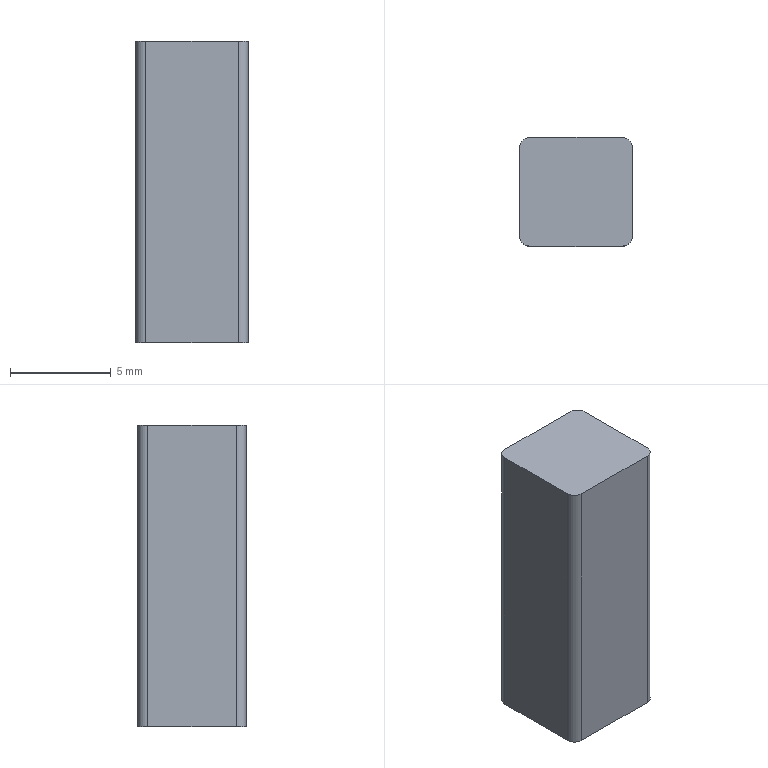Part | NX | features BREP 1 | 1 solid | 10 faces | box 5.6 x 5.4 x 15 mm | volume 450.381 mm3 | plane 6 | cylinder 4 | commonest cylinder face diameters 1 x4
STEP:
#1=CARTESIAN_POINT('',(-2.3,2.7,-25.6));
#2=VERTEX_POINT('',#1);
#3=CARTESIAN_POINT('',(-2.8,2.2,-25.6));
#4=VERTEX_POINT('',#3);
#5=CARTESIAN_POINT('',(-2.3,2.2,-25.6));
#6=DIRECTION('',(0.,0.,1.));
#7=DIRECTION('',(1.,0.,0.));
#8=AXIS2_PLACEMENT_3D('',#5,#6,#7);
#9=CIRCLE('',#8,0.5);
#10=EDGE_CURVE('',#2,#4,#9,.T.);
#11=ORIENTED_EDGE('',*,*,#10,.F.);
#12=CARTESIAN_POINT('',(-2.3,2.7,-40.6));
#13=VERTEX_POINT('',#12);
#14=CARTESIAN_POINT('',(-2.3,2.7,-40.6));
#15=DIRECTION('',(0.,0.,1.));
#16=VECTOR('',#15,1000.);
#17=LINE('',#14,#16);
#18=EDGE_CURVE('',#13,#2,#17,.T.);
#19=ORIENTED_EDGE('',*,*,#18,.F.);
#20=CARTESIAN_POINT('',(-2.8,2.2,-40.6));
#21=VERTEX_POINT('',#20);
#22=CARTESIAN_POINT('',(-2.3,2.2,-40.6));
#23=DIRECTION('',(0.,0.,1.));
#24=DIRECTION('',(1.,0.,0.));
#25=AXIS2_PLACEMENT_3D('',#22,#23,#24);
#26=CIRCLE('',#25,0.5);
#27=EDGE_CURVE('',#13,#21,#26,.T.);
#28=ORIENTED_EDGE('',*,*,#27,.T.);
#29=CARTESIAN_POINT('',(-2.8,2.2,-40.6));
#30=DIRECTION('',(0.,0.,1.));
#31=VECTOR('',#30,1000.);
#32=LINE('',#29,#31);
#33=EDGE_CURVE('',#21,#4,#32,.T.);
#34=ORIENTED_EDGE('',*,*,#33,.T.);
#35=EDGE_LOOP('',(#11,#19,#28,#34));
#36=FACE_BOUND('',#35,.T.);
#37=CARTESIAN_POINT('',(-2.3,2.2,-40.6));
#38=DIRECTION('',(0.,0.,1.));
#39=DIRECTION('',(-1.,0.,0.));
#40=AXIS2_PLACEMENT_3D('',#37,#38,#39);
#41=CYLINDRICAL_SURFACE('',#40,0.5);
#42=ADVANCED_FACE('',(#36),#41,.T.);
#43=CARTESIAN_POINT('',(-2.8,-2.2,-25.6));
#44=VERTEX_POINT('',#43);
#45=CARTESIAN_POINT('',(-2.8,-2.2,-25.6));
#46=DIRECTION('',(0.,1.,0.));
#47=VECTOR('',#46,1000.);
#48=LINE('',#45,#47);
#49=EDGE_CURVE('',#44,#4,#48,.T.);
#50=ORIENTED_EDGE('',*,*,#49,.T.);
#51=ORIENTED_EDGE('',*,*,#33,.F.);
#52=CARTESIAN_POINT('',(-2.8,-2.2,-40.6));
#53=VERTEX_POINT('',#52);
#54=CARTESIAN_POINT('',(-2.8,-2.2,-40.6));
#55=DIRECTION('',(0.,1.,0.));
#56=VECTOR('',#55,1000.);
#57=LINE('',#54,#56);
#58=EDGE_CURVE('',#53,#21,#57,.T.);
#59=ORIENTED_EDGE('',*,*,#58,.F.);
#60=CARTESIAN_POINT('',(-2.8,-2.2,-40.6));
#61=DIRECTION('',(0.,0.,1.));
#62=VECTOR('',#61,1000.);
#63=LINE('',#60,#62);
#64=EDGE_CURVE('',#53,#44,#63,.T.);
#65=ORIENTED_EDGE('',*,*,#64,.T.);
#66=EDGE_LOOP('',(#50,#51,#59,#65));
#67=FACE_BOUND('',#66,.T.);
#68=CARTESIAN_POINT('',(-2.8,-2.2,-40.6));
#69=DIRECTION('',(1.,0.,0.));
#70=DIRECTION('',(0.,0.,1.));
#71=AXIS2_PLACEMENT_3D('',#68,#69,#70);
#72=PLANE('',#71);
#73=ADVANCED_FACE('',(#67),#72,.F.);
#74=CARTESIAN_POINT('',(-2.3,-2.7,-25.6));
#75=VERTEX_POINT('',#74);
#76=CARTESIAN_POINT('',(-2.3,-2.2,-25.6));
#77=DIRECTION('',(0.,0.,1.));
#78=DIRECTION('',(1.,0.,0.));
#79=AXIS2_PLACEMENT_3D('',#76,#77,#78);
#80=CIRCLE('',#79,0.5);
#81=EDGE_CURVE('',#44,#75,#80,.T.);
#82=ORIENTED_EDGE('',*,*,#81,.F.);
#83=ORIENTED_EDGE('',*,*,#64,.F.);
#84=CARTESIAN_POINT('',(-2.3,-2.7,-40.6));
#85=VERTEX_POINT('',#84);
#86=CARTESIAN_POINT('',(-2.3,-2.2,-40.6));
#87=DIRECTION('',(0.,0.,1.));
#88=DIRECTION('',(1.,0.,0.));
#89=AXIS2_PLACEMENT_3D('',#86,#87,#88);
#90=CIRCLE('',#89,0.5);
#91=EDGE_CURVE('',#53,#85,#90,.T.);
#92=ORIENTED_EDGE('',*,*,#91,.T.);
#93=CARTESIAN_POINT('',(-2.3,-2.7,-40.6));
#94=DIRECTION('',(0.,0.,1.));
#95=VECTOR('',#94,1000.);
#96=LINE('',#93,#95);
#97=EDGE_CURVE('',#85,#75,#96,.T.);
#98=ORIENTED_EDGE('',*,*,#97,.T.);
#99=EDGE_LOOP('',(#82,#83,#92,#98));
#100=FACE_BOUND('',#99,.T.);
#101=CARTESIAN_POINT('',(-2.3,-2.2,-40.6));
#102=DIRECTION('',(0.,0.,1.));
#103=DIRECTION('',(-1.,0.,0.));
#104=AXIS2_PLACEMENT_3D('',#101,#102,#103);
#105=CYLINDRICAL_SURFACE('',#104,0.5);
#106=ADVANCED_FACE('',(#100),#105,.T.);
#107=CARTESIAN_POINT('',(2.3,-2.7,-25.6));
#108=VERTEX_POINT('',#107);
#109=CARTESIAN_POINT('',(2.3,-2.7,-25.6));
#110=DIRECTION('',(-1.,0.,0.));
#111=VECTOR('',#110,1000.);
#112=LINE('',#109,#111);
#113=EDGE_CURVE('',#108,#75,#112,.T.);
#114=ORIENTED_EDGE('',*,*,#113,.T.);
#115=ORIENTED_EDGE('',*,*,#97,.F.);
#116=CARTESIAN_POINT('',(2.3,-2.7,-40.6));
#117=VERTEX_POINT('',#116);
#118=CARTESIAN_POINT('',(2.3,-2.7,-40.6));
#119=DIRECTION('',(-1.,0.,0.));
#120=VECTOR('',#119,1000.);
#121=LINE('',#118,#120);
#122=EDGE_CURVE('',#117,#85,#121,.T.);
#123=ORIENTED_EDGE('',*,*,#122,.F.);
#124=CARTESIAN_POINT('',(2.3,-2.7,-40.6));
#125=DIRECTION('',(0.,0.,1.));
#126=VECTOR('',#125,1000.);
#127=LINE('',#124,#126);
#128=EDGE_CURVE('',#117,#108,#127,.T.);
#129=ORIENTED_EDGE('',*,*,#128,.T.);
#130=EDGE_LOOP('',(#114,#115,#123,#129));
#131=FACE_BOUND('',#130,.T.);
#132=CARTESIAN_POINT('',(2.3,-2.7,-40.6));
#133=DIRECTION('',(0.,1.,0.));
#134=DIRECTION('',(0.,0.,-1.));
#135=AXIS2_PLACEMENT_3D('',#132,#133,#134);
#136=PLANE('',#135);
#137=ADVANCED_FACE('',(#131),#136,.F.);
#138=CARTESIAN_POINT('',(2.8,-2.2,-25.6));
#139=VERTEX_POINT('',#138);
#140=CARTESIAN_POINT('',(2.3,-2.2,-25.6));
#141=DIRECTION('',(0.,0.,1.));
#142=DIRECTION('',(1.,0.,0.));
#143=AXIS2_PLACEMENT_3D('',#140,#141,#142);
#144=CIRCLE('',#143,0.5);
#145=EDGE_CURVE('',#108,#139,#144,.T.);
#146=ORIENTED_EDGE('',*,*,#145,.F.);
#147=ORIENTED_EDGE('',*,*,#128,.F.);
#148=CARTESIAN_POINT('',(2.8,-2.2,-40.6));
#149=VERTEX_POINT('',#148);
#150=CARTESIAN_POINT('',(2.3,-2.2,-40.6));
#151=DIRECTION('',(0.,0.,1.));
#152=DIRECTION('',(1.,0.,0.));
#153=AXIS2_PLACEMENT_3D('',#150,#151,#152);
#154=CIRCLE('',#153,0.5);
#155=EDGE_CURVE('',#117,#149,#154,.T.);
#156=ORIENTED_EDGE('',*,*,#155,.T.);
#157=CARTESIAN_POINT('',(2.8,-2.2,-40.6));
#158=DIRECTION('',(0.,0.,1.));
#159=VECTOR('',#158,1000.);
#160=LINE('',#157,#159);
#161=EDGE_CURVE('',#149,#139,#160,.T.);
#162=ORIENTED_EDGE('',*,*,#161,.T.);
#163=EDGE_LOOP('',(#146,#147,#156,#162));
#164=FACE_BOUND('',#163,.T.);
#165=CARTESIAN_POINT('',(2.3,-2.2,-40.6));
#166=DIRECTION('',(0.,0.,1.));
#167=DIRECTION('',(-1.,0.,0.));
#168=AXIS2_PLACEMENT_3D('',#165,#166,#167);
#169=CYLINDRICAL_SURFACE('',#168,0.5);
#170=ADVANCED_FACE('',(#164),#169,.T.);
#171=CARTESIAN_POINT('',(2.8,2.2,-25.6));
#172=VERTEX_POINT('',#171);
#173=CARTESIAN_POINT('',(2.8,2.2,-25.6));
#174=DIRECTION('',(0.,-1.,0.));
#175=VECTOR('',#174,1000.);
#176=LINE('',#173,#175);
#177=EDGE_CURVE('',#172,#139,#176,.T.);
#178=ORIENTED_EDGE('',*,*,#177,.T.);
#179=ORIENTED_EDGE('',*,*,#161,.F.);
#180=CARTESIAN_POINT('',(2.8,2.2,-40.6));
#181=VERTEX_POINT('',#180);
#182=CARTESIAN_POINT('',(2.8,2.2,-40.6));
#183=DIRECTION('',(0.,-1.,0.));
#184=VECTOR('',#183,1000.);
#185=LINE('',#182,#184);
#186=EDGE_CURVE('',#181,#149,#185,.T.);
#187=ORIENTED_EDGE('',*,*,#186,.F.);
#188=CARTESIAN_POINT('',(2.8,2.2,-40.6));
#189=DIRECTION('',(0.,0.,1.));
#190=VECTOR('',#189,1000.);
#191=LINE('',#188,#190);
#192=EDGE_CURVE('',#181,#172,#191,.T.);
#193=ORIENTED_EDGE('',*,*,#192,.T.);
#194=EDGE_LOOP('',(#178,#179,#187,#193));
#195=FACE_BOUND('',#194,.T.);
#196=CARTESIAN_POINT('',(2.8,2.2,-40.6));
#197=DIRECTION('',(-1.,0.,0.));
#198=DIRECTION('',(0.,0.,-1.));
#199=AXIS2_PLACEMENT_3D('',#196,#197,#198);
#200=PLANE('',#199);
#201=ADVANCED_FACE('',(#195),#200,.F.);
#202=CARTESIAN_POINT('',(2.3,2.7,-25.6));
#203=VERTEX_POINT('',#202);
#204=CARTESIAN_POINT('',(2.3,2.2,-25.6));
#205=DIRECTION('',(0.,0.,1.));
#206=DIRECTION('',(1.,0.,0.));
#207=AXIS2_PLACEMENT_3D('',#204,#205,#206);
#208=CIRCLE('',#207,0.5);
#209=EDGE_CURVE('',#172,#203,#208,.T.);
#210=ORIENTED_EDGE('',*,*,#209,.F.);
#211=ORIENTED_EDGE('',*,*,#192,.F.);
#212=CARTESIAN_POINT('',(2.3,2.7,-40.6));
#213=VERTEX_POINT('',#212);
#214=CARTESIAN_POINT('',(2.3,2.2,-40.6));
#215=DIRECTION('',(0.,0.,1.));
#216=DIRECTION('',(1.,0.,0.));
#217=AXIS2_PLACEMENT_3D('',#214,#215,#216);
#218=CIRCLE('',#217,0.5);
#219=EDGE_CURVE('',#181,#213,#218,.T.);
#220=ORIENTED_EDGE('',*,*,#219,.T.);
#221=CARTESIAN_POINT('',(2.3,2.7,-40.6));
#222=DIRECTION('',(0.,0.,1.));
#223=VECTOR('',#222,1000.);
#224=LINE('',#221,#223);
#225=EDGE_CURVE('',#213,#203,#224,.T.);
#226=ORIENTED_EDGE('',*,*,#225,.T.);
#227=EDGE_LOOP('',(#210,#211,#220,#226));
#228=FACE_BOUND('',#227,.T.);
#229=CARTESIAN_POINT('',(2.3,2.2,-40.6));
#230=DIRECTION('',(0.,0.,1.));
#231=DIRECTION('',(-1.,0.,0.));
#232=AXIS2_PLACEMENT_3D('',#229,#230,#231);
#233=CYLINDRICAL_SURFACE('',#232,0.5);
#234=ADVANCED_FACE('',(#228),#233,.T.);
#235=CARTESIAN_POINT('',(-2.3,2.7,-25.6));
#236=DIRECTION('',(1.,0.,0.));
#237=VECTOR('',#236,1000.);
#238=LINE('',#235,#237);
#239=EDGE_CURVE('',#2,#203,#238,.T.);
#240=ORIENTED_EDGE('',*,*,#239,.T.);
#241=ORIENTED_EDGE('',*,*,#225,.F.);
#242=CARTESIAN_POINT('',(-2.3,2.7,-40.6));
#243=DIRECTION('',(1.,0.,0.));
#244=VECTOR('',#243,1000.);
#245=LINE('',#242,#244);
#246=EDGE_CURVE('',#13,#213,#245,.T.);
#247=ORIENTED_EDGE('',*,*,#246,.F.);
#248=ORIENTED_EDGE('',*,*,#18,.T.);
#249=EDGE_LOOP('',(#240,#241,#247,#248));
#250=FACE_BOUND('',#249,.T.);
#251=CARTESIAN_POINT('',(-2.3,2.7,-40.6));
#252=DIRECTION('',(0.,-1.,0.));
#253=DIRECTION('',(0.,0.,1.));
#254=AXIS2_PLACEMENT_3D('',#251,#252,#253);
#255=PLANE('',#254);
#256=ADVANCED_FACE('',(#250),#255,.F.);
#257=ORIENTED_EDGE('',*,*,#27,.F.);
#258=ORIENTED_EDGE('',*,*,#246,.T.);
#259=ORIENTED_EDGE('',*,*,#219,.F.);
#260=ORIENTED_EDGE('',*,*,#186,.T.);
#261=ORIENTED_EDGE('',*,*,#155,.F.);
#262=ORIENTED_EDGE('',*,*,#122,.T.);
#263=ORIENTED_EDGE('',*,*,#91,.F.);
#264=ORIENTED_EDGE('',*,*,#58,.T.);
#265=EDGE_LOOP('',(#257,#258,#259,#260,#261,#262,#263,#264));
#266=FACE_BOUND('',#265,.T.);
#267=CARTESIAN_POINT('',(-2.3,2.2,-40.6));
#268=DIRECTION('',(0.,0.,1.));
#269=DIRECTION('',(-1.,0.,0.));
#270=AXIS2_PLACEMENT_3D('',#267,#268,#269);
#271=PLANE('',#270);
#272=ADVANCED_FACE('',(#266),#271,.F.);
#273=ORIENTED_EDGE('',*,*,#10,.T.);
#274=ORIENTED_EDGE('',*,*,#49,.F.);
#275=ORIENTED_EDGE('',*,*,#81,.T.);
#276=ORIENTED_EDGE('',*,*,#113,.F.);
#277=ORIENTED_EDGE('',*,*,#145,.T.);
#278=ORIENTED_EDGE('',*,*,#177,.F.);
#279=ORIENTED_EDGE('',*,*,#209,.T.);
#280=ORIENTED_EDGE('',*,*,#239,.F.);
#281=EDGE_LOOP('',(#273,#274,#275,#276,#277,#278,#279,#280));
#282=FACE_BOUND('',#281,.T.);
#283=CARTESIAN_POINT('',(-2.3,2.2,-25.6));
#284=DIRECTION('',(0.,0.,1.));
#285=DIRECTION('',(-1.,0.,0.));
#286=AXIS2_PLACEMENT_3D('',#283,#284,#285);
#287=PLANE('',#286);
#288=ADVANCED_FACE('',(#282),#287,.T.);
#289=CLOSED_SHELL('',(#42,#73,#106,#137,#170,#201,#234,#256,#272,#288));
#290=MANIFOLD_SOLID_BREP('',#289);
#291=(LENGTH_UNIT()NAMED_UNIT(*)SI_UNIT(.MILLI.,.METRE.));
#292=UNCERTAINTY_MEASURE_WITH_UNIT(LENGTH_MEASURE(0.00001),#291,'','');
#293=(NAMED_UNIT(*)PLANE_ANGLE_UNIT()SI_UNIT($,.RADIAN.));
#294=(NAMED_UNIT(*)SI_UNIT($,.STERADIAN.)SOLID_ANGLE_UNIT());
#295=(GEOMETRIC_REPRESENTATION_CONTEXT(3)GLOBAL_UNCERTAINTY_ASSIGNED_CONTEXT((#292))GLOBAL_UNIT_ASSIGNED_CONTEXT((#291,#293,#294))REPRESENTATION_CONTEXT('',''));
#296=ADVANCED_BREP_SHAPE_REPRESENTATION('',(#290),#295);